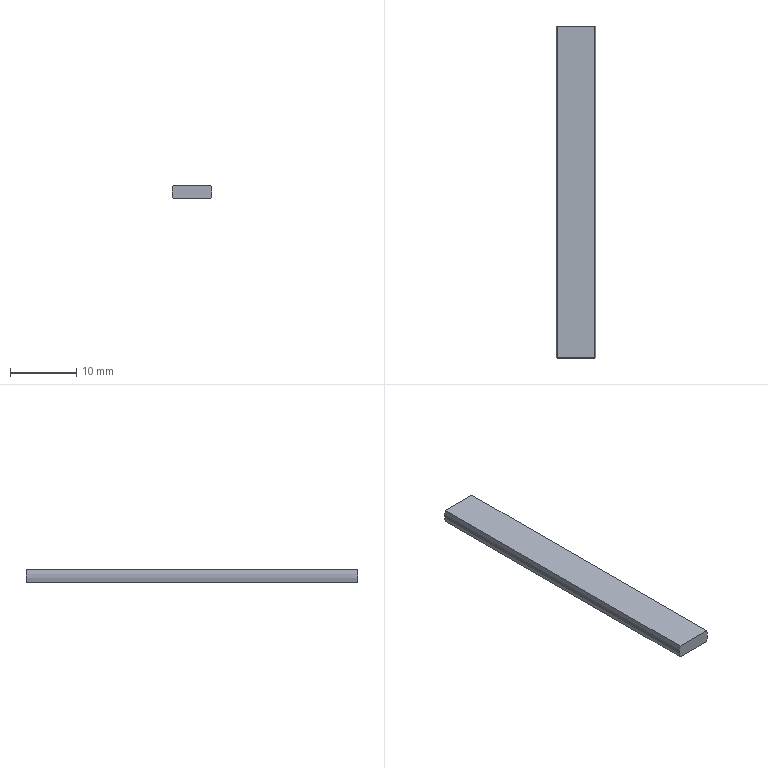Part | STEP file | Cooling fin - Tower - 1 cav | 1 solid | 6 faces | box 6 x 50 x 2 mm | volume 588.696 mm3 | plane 4 | cylinder 2 | commonest cylinder face diameters 6 x2
STEP:
#1=CARTESIAN_POINT('',(0.,0.,0.));
#2=DIRECTION('',(0.,0.,1.));
#3=DIRECTION('',(1.,0.,0.));
#4=AXIS2_PLACEMENT_3D('',#1,#2,#3);
#5=CARTESIAN_POINT('',(2.828,0.,-1.));
#6=VERTEX_POINT('',#5);
#7=CARTESIAN_POINT('',(2.828,50.,-1.));
#8=VERTEX_POINT('',#7);
#9=CARTESIAN_POINT('',(2.828,0.,-1.));
#10=DIRECTION('',(0.,1.,0.));
#11=VECTOR('',#10,1.);
#12=LINE('',#9,#11);
#13=CARTESIAN_POINT('',(-5.,50.,-1.));
#14=DIRECTION('',(0.,0.,1.));
#15=DIRECTION('',(1.,0.,0.));
#16=AXIS2_PLACEMENT_3D('',#13,#14,#15);
#17=PLANE('',#16);
#18=CARTESIAN_POINT('',(7.828,-50.));
#19=DIRECTION('',(0.,1.));
#20=VECTOR('',#19,1.);
#21=LINE('',#18,#20);
#22=(GEOMETRIC_REPRESENTATION_CONTEXT(2)PARAMETRIC_REPRESENTATION_CONTEXT()REPRESENTATION_CONTEXT('',''));
#23=DEFINITIONAL_REPRESENTATION('',(#21),#22);
#24=PCURVE('',#17,#23);
#25=CARTESIAN_POINT('',(0.,0.,0.));
#26=DIRECTION('',(0.,1.,0.));
#27=DIRECTION('',(0.,0.,1.));
#28=AXIS2_PLACEMENT_3D('',#25,#26,#27);
#29=CYLINDRICAL_SURFACE('',#28,3.);
#30=CARTESIAN_POINT('',(1.911,0.));
#31=DIRECTION('',(0.,1.));
#32=VECTOR('',#31,1.);
#33=LINE('',#30,#32);
#34=(GEOMETRIC_REPRESENTATION_CONTEXT(2)PARAMETRIC_REPRESENTATION_CONTEXT()REPRESENTATION_CONTEXT('',''));
#35=DEFINITIONAL_REPRESENTATION('',(#33),#34);
#36=PCURVE('',#29,#35);
#37=SURFACE_CURVE('',#12,(#24,#36),.PCURVE_S1.);
#38=EDGE_CURVE('',#6,#8,#37,.T.);
#39=ORIENTED_EDGE('',*,*,#38,.F.);
#40=CARTESIAN_POINT('',(-2.828,0.,-1.));
#41=VERTEX_POINT('',#40);
#42=CARTESIAN_POINT('',(-5.,0.,-1.));
#43=DIRECTION('',(-1.,0.,0.));
#44=VECTOR('',#43,1.);
#45=LINE('',#42,#44);
#46=CARTESIAN_POINT('',(0.,-50.));
#47=DIRECTION('',(-1.,0.));
#48=VECTOR('',#47,1.);
#49=LINE('',#46,#48);
#50=(GEOMETRIC_REPRESENTATION_CONTEXT(2)PARAMETRIC_REPRESENTATION_CONTEXT()REPRESENTATION_CONTEXT('',''));
#51=DEFINITIONAL_REPRESENTATION('',(#49),#50);
#52=PCURVE('',#17,#51);
#53=CARTESIAN_POINT('',(0.,0.,0.));
#54=DIRECTION('',(0.,-1.,0.));
#55=DIRECTION('',(0.,0.,-1.));
#56=AXIS2_PLACEMENT_3D('',#53,#54,#55);
#57=PLANE('',#56);
#58=CARTESIAN_POINT('',(1.,-5.));
#59=DIRECTION('',(0.,-1.));
#60=VECTOR('',#59,1.);
#61=LINE('',#58,#60);
#62=(GEOMETRIC_REPRESENTATION_CONTEXT(2)PARAMETRIC_REPRESENTATION_CONTEXT()REPRESENTATION_CONTEXT('',''));
#63=DEFINITIONAL_REPRESENTATION('',(#61),#62);
#64=PCURVE('',#57,#63);
#65=SURFACE_CURVE('',#45,(#52,#64),.PCURVE_S1.);
#66=EDGE_CURVE('',#6,#41,#65,.T.);
#67=ORIENTED_EDGE('',*,*,#66,.T.);
#68=CARTESIAN_POINT('',(-2.828,50.,-1.));
#69=VERTEX_POINT('',#68);
#70=CARTESIAN_POINT('',(-2.828,0.,-1.));
#71=DIRECTION('',(0.,-1.,0.));
#72=VECTOR('',#71,1.);
#73=LINE('',#70,#72);
#74=CARTESIAN_POINT('',(2.172,-50.));
#75=DIRECTION('',(0.,-1.));
#76=VECTOR('',#75,1.);
#77=LINE('',#74,#76);
#78=(GEOMETRIC_REPRESENTATION_CONTEXT(2)PARAMETRIC_REPRESENTATION_CONTEXT()REPRESENTATION_CONTEXT('',''));
#79=DEFINITIONAL_REPRESENTATION('',(#77),#78);
#80=PCURVE('',#17,#79);
#81=CARTESIAN_POINT('',(0.,0.,0.));
#82=DIRECTION('',(0.,1.,0.));
#83=DIRECTION('',(0.,0.,1.));
#84=AXIS2_PLACEMENT_3D('',#81,#82,#83);
#85=CYLINDRICAL_SURFACE('',#84,3.);
#86=CARTESIAN_POINT('',(4.373,0.));
#87=DIRECTION('',(0.,-1.));
#88=VECTOR('',#87,1.);
#89=LINE('',#86,#88);
#90=(GEOMETRIC_REPRESENTATION_CONTEXT(2)PARAMETRIC_REPRESENTATION_CONTEXT()REPRESENTATION_CONTEXT('',''));
#91=DEFINITIONAL_REPRESENTATION('',(#89),#90);
#92=PCURVE('',#85,#91);
#93=SURFACE_CURVE('',#73,(#80,#92),.PCURVE_S1.);
#94=EDGE_CURVE('',#69,#41,#93,.T.);
#95=ORIENTED_EDGE('',*,*,#94,.F.);
#96=CARTESIAN_POINT('',(-5.,50.,-1.));
#97=DIRECTION('',(-1.,0.,0.));
#98=VECTOR('',#97,1.);
#99=LINE('',#96,#98);
#100=CARTESIAN_POINT('',(0.,0.));
#101=DIRECTION('',(-1.,0.));
#102=VECTOR('',#101,1.);
#103=LINE('',#100,#102);
#104=(GEOMETRIC_REPRESENTATION_CONTEXT(2)PARAMETRIC_REPRESENTATION_CONTEXT()REPRESENTATION_CONTEXT('',''));
#105=DEFINITIONAL_REPRESENTATION('',(#103),#104);
#106=PCURVE('',#17,#105);
#107=CARTESIAN_POINT('',(0.,50.,0.));
#108=DIRECTION('',(0.,-1.,0.));
#109=DIRECTION('',(0.,0.,-1.));
#110=AXIS2_PLACEMENT_3D('',#107,#108,#109);
#111=PLANE('',#110);
#112=CARTESIAN_POINT('',(1.,-5.));
#113=DIRECTION('',(0.,-1.));
#114=VECTOR('',#113,1.);
#115=LINE('',#112,#114);
#116=(GEOMETRIC_REPRESENTATION_CONTEXT(2)PARAMETRIC_REPRESENTATION_CONTEXT()REPRESENTATION_CONTEXT('',''));
#117=DEFINITIONAL_REPRESENTATION('',(#115),#116);
#118=PCURVE('',#111,#117);
#119=SURFACE_CURVE('',#99,(#106,#118),.PCURVE_S1.);
#120=EDGE_CURVE('',#8,#69,#119,.T.);
#121=ORIENTED_EDGE('',*,*,#120,.F.);
#122=EDGE_LOOP('',(#39,#67,#95,#121));
#123=FACE_BOUND('',#122,.T.);
#124=ADVANCED_FACE('',(#123),#17,.F.);
#125=CARTESIAN_POINT('',(-2.828,0.,1.));
#126=VERTEX_POINT('',#125);
#127=CARTESIAN_POINT('',(-2.828,50.,1.));
#128=VERTEX_POINT('',#127);
#129=CARTESIAN_POINT('',(-2.828,0.,1.));
#130=DIRECTION('',(0.,1.,0.));
#131=VECTOR('',#130,1.);
#132=LINE('',#129,#131);
#133=CARTESIAN_POINT('',(-5.,50.,1.));
#134=DIRECTION('',(0.,0.,-1.));
#135=DIRECTION('',(-1.,0.,0.));
#136=AXIS2_PLACEMENT_3D('',#133,#134,#135);
#137=PLANE('',#136);
#138=CARTESIAN_POINT('',(-2.172,-50.));
#139=DIRECTION('',(0.,1.));
#140=VECTOR('',#139,1.);
#141=LINE('',#138,#140);
#142=(GEOMETRIC_REPRESENTATION_CONTEXT(2)PARAMETRIC_REPRESENTATION_CONTEXT()REPRESENTATION_CONTEXT('',''));
#143=DEFINITIONAL_REPRESENTATION('',(#141),#142);
#144=PCURVE('',#137,#143);
#145=CARTESIAN_POINT('',(5.052,0.));
#146=DIRECTION('',(0.,1.));
#147=VECTOR('',#146,1.);
#148=LINE('',#145,#147);
#149=(GEOMETRIC_REPRESENTATION_CONTEXT(2)PARAMETRIC_REPRESENTATION_CONTEXT()REPRESENTATION_CONTEXT('',''));
#150=DEFINITIONAL_REPRESENTATION('',(#148),#149);
#151=PCURVE('',#85,#150);
#152=SURFACE_CURVE('',#132,(#144,#151),.PCURVE_S1.);
#153=EDGE_CURVE('',#126,#128,#152,.T.);
#154=ORIENTED_EDGE('',*,*,#153,.F.);
#155=CARTESIAN_POINT('',(2.828,0.,1.));
#156=VERTEX_POINT('',#155);
#157=CARTESIAN_POINT('',(-5.,0.,1.));
#158=DIRECTION('',(1.,0.,0.));
#159=VECTOR('',#158,1.);
#160=LINE('',#157,#159);
#161=CARTESIAN_POINT('',(0.,-50.));
#162=DIRECTION('',(-1.,0.));
#163=VECTOR('',#162,1.);
#164=LINE('',#161,#163);
#165=(GEOMETRIC_REPRESENTATION_CONTEXT(2)PARAMETRIC_REPRESENTATION_CONTEXT()REPRESENTATION_CONTEXT('',''));
#166=DEFINITIONAL_REPRESENTATION('',(#164),#165);
#167=PCURVE('',#137,#166);
#168=CARTESIAN_POINT('',(-1.,-5.));
#169=DIRECTION('',(0.,1.));
#170=VECTOR('',#169,1.);
#171=LINE('',#168,#170);
#172=(GEOMETRIC_REPRESENTATION_CONTEXT(2)PARAMETRIC_REPRESENTATION_CONTEXT()REPRESENTATION_CONTEXT('',''));
#173=DEFINITIONAL_REPRESENTATION('',(#171),#172);
#174=PCURVE('',#57,#173);
#175=SURFACE_CURVE('',#160,(#167,#174),.PCURVE_S1.);
#176=EDGE_CURVE('',#126,#156,#175,.T.);
#177=ORIENTED_EDGE('',*,*,#176,.T.);
#178=CARTESIAN_POINT('',(2.828,50.,1.));
#179=VERTEX_POINT('',#178);
#180=CARTESIAN_POINT('',(2.828,0.,1.));
#181=DIRECTION('',(0.,-1.,0.));
#182=VECTOR('',#181,1.);
#183=LINE('',#180,#182);
#184=CARTESIAN_POINT('',(-7.828,-50.));
#185=DIRECTION('',(0.,-1.));
#186=VECTOR('',#185,1.);
#187=LINE('',#184,#186);
#188=(GEOMETRIC_REPRESENTATION_CONTEXT(2)PARAMETRIC_REPRESENTATION_CONTEXT()REPRESENTATION_CONTEXT('',''));
#189=DEFINITIONAL_REPRESENTATION('',(#187),#188);
#190=PCURVE('',#137,#189);
#191=CARTESIAN_POINT('',(1.231,0.));
#192=DIRECTION('',(0.,-1.));
#193=VECTOR('',#192,1.);
#194=LINE('',#191,#193);
#195=(GEOMETRIC_REPRESENTATION_CONTEXT(2)PARAMETRIC_REPRESENTATION_CONTEXT()REPRESENTATION_CONTEXT('',''));
#196=DEFINITIONAL_REPRESENTATION('',(#194),#195);
#197=PCURVE('',#29,#196);
#198=SURFACE_CURVE('',#183,(#190,#197),.PCURVE_S1.);
#199=EDGE_CURVE('',#179,#156,#198,.T.);
#200=ORIENTED_EDGE('',*,*,#199,.F.);
#201=CARTESIAN_POINT('',(-5.,50.,1.));
#202=DIRECTION('',(1.,0.,0.));
#203=VECTOR('',#202,1.);
#204=LINE('',#201,#203);
#205=CARTESIAN_POINT('',(0.,0.));
#206=DIRECTION('',(-1.,0.));
#207=VECTOR('',#206,1.);
#208=LINE('',#205,#207);
#209=(GEOMETRIC_REPRESENTATION_CONTEXT(2)PARAMETRIC_REPRESENTATION_CONTEXT()REPRESENTATION_CONTEXT('',''));
#210=DEFINITIONAL_REPRESENTATION('',(#208),#209);
#211=PCURVE('',#137,#210);
#212=CARTESIAN_POINT('',(-1.,-5.));
#213=DIRECTION('',(0.,1.));
#214=VECTOR('',#213,1.);
#215=LINE('',#212,#214);
#216=(GEOMETRIC_REPRESENTATION_CONTEXT(2)PARAMETRIC_REPRESENTATION_CONTEXT()REPRESENTATION_CONTEXT('',''));
#217=DEFINITIONAL_REPRESENTATION('',(#215),#216);
#218=PCURVE('',#111,#217);
#219=SURFACE_CURVE('',#204,(#211,#218),.PCURVE_S1.);
#220=EDGE_CURVE('',#128,#179,#219,.T.);
#221=ORIENTED_EDGE('',*,*,#220,.F.);
#222=EDGE_LOOP('',(#154,#177,#200,#221));
#223=FACE_BOUND('',#222,.T.);
#224=ADVANCED_FACE('',(#223),#137,.F.);
#225=CARTESIAN_POINT('',(0.,50.,0.));
#226=DIRECTION('',(0.,1.,0.));
#227=DIRECTION('',(0.,0.,1.));
#228=AXIS2_PLACEMENT_3D('',#225,#226,#227);
#229=CIRCLE('',#228,3.);
#230=CARTESIAN_POINT('',(-3.,0.));
#231=CARTESIAN_POINT('',(-3.,5.196));
#232=CARTESIAN_POINT('',(1.5,2.598));
#233=CARTESIAN_POINT('',(6.,0.));
#234=CARTESIAN_POINT('',(1.5,-2.598));
#235=CARTESIAN_POINT('',(-3.,-5.196));
#236=CARTESIAN_POINT('',(-3.,0.));
#237=(BOUNDED_CURVE()B_SPLINE_CURVE(2,(#230,#231,#232,#233,#234,#235,#236),.UNSPECIFIED.,.T.,.F.)B_SPLINE_CURVE_WITH_KNOTS((1,2,2,2,2,1),(-2.094,0.,2.094,4.189,6.283,8.378),.UNSPECIFIED.)CURVE()GEOMETRIC_REPRESENTATION_ITEM()RATIONAL_B_SPLINE_CURVE((1.,0.5,1.,0.5,1.,0.5,1.))REPRESENTATION_ITEM(''));
#238=(GEOMETRIC_REPRESENTATION_CONTEXT(2)PARAMETRIC_REPRESENTATION_CONTEXT()REPRESENTATION_CONTEXT('',''));
#239=DEFINITIONAL_REPRESENTATION('',(#237),#238);
#240=PCURVE('',#111,#239);
#241=CARTESIAN_POINT('',(0.,50.));
#242=DIRECTION('',(1.,0.));
#243=VECTOR('',#242,1.);
#244=LINE('',#241,#243);
#245=(GEOMETRIC_REPRESENTATION_CONTEXT(2)PARAMETRIC_REPRESENTATION_CONTEXT()REPRESENTATION_CONTEXT('',''));
#246=DEFINITIONAL_REPRESENTATION('',(#244),#245);
#247=PCURVE('',#29,#246);
#248=SURFACE_CURVE('',#229,(#240,#247),.PCURVE_S1.);
#249=EDGE_CURVE('',#179,#8,#248,.T.);
#250=ORIENTED_EDGE('',*,*,#249,.T.);
#251=ORIENTED_EDGE('',*,*,#120,.T.);
#252=CARTESIAN_POINT('',(0.,50.,0.));
#253=DIRECTION('',(0.,1.,0.));
#254=DIRECTION('',(0.,0.,1.));
#255=AXIS2_PLACEMENT_3D('',#252,#253,#254);
#256=CIRCLE('',#255,3.);
#257=CARTESIAN_POINT('',(-3.,0.));
#258=CARTESIAN_POINT('',(-3.,5.196));
#259=CARTESIAN_POINT('',(1.5,2.598));
#260=CARTESIAN_POINT('',(6.,0.));
#261=CARTESIAN_POINT('',(1.5,-2.598));
#262=CARTESIAN_POINT('',(-3.,-5.196));
#263=CARTESIAN_POINT('',(-3.,0.));
#264=(BOUNDED_CURVE()B_SPLINE_CURVE(2,(#257,#258,#259,#260,#261,#262,#263),.UNSPECIFIED.,.T.,.F.)B_SPLINE_CURVE_WITH_KNOTS((1,2,2,2,2,1),(-2.094,0.,2.094,4.189,6.283,8.378),.UNSPECIFIED.)CURVE()GEOMETRIC_REPRESENTATION_ITEM()RATIONAL_B_SPLINE_CURVE((1.,0.5,1.,0.5,1.,0.5,1.))REPRESENTATION_ITEM(''));
#265=(GEOMETRIC_REPRESENTATION_CONTEXT(2)PARAMETRIC_REPRESENTATION_CONTEXT()REPRESENTATION_CONTEXT('',''));
#266=DEFINITIONAL_REPRESENTATION('',(#264),#265);
#267=PCURVE('',#111,#266);
#268=CARTESIAN_POINT('',(0.,50.));
#269=DIRECTION('',(1.,0.));
#270=VECTOR('',#269,1.);
#271=LINE('',#268,#270);
#272=(GEOMETRIC_REPRESENTATION_CONTEXT(2)PARAMETRIC_REPRESENTATION_CONTEXT()REPRESENTATION_CONTEXT('',''));
#273=DEFINITIONAL_REPRESENTATION('',(#271),#272);
#274=PCURVE('',#85,#273);
#275=SURFACE_CURVE('',#256,(#267,#274),.PCURVE_S1.);
#276=EDGE_CURVE('',#69,#128,#275,.T.);
#277=ORIENTED_EDGE('',*,*,#276,.T.);
#278=ORIENTED_EDGE('',*,*,#220,.T.);
#279=EDGE_LOOP('',(#250,#251,#277,#278));
#280=FACE_BOUND('',#279,.T.);
#281=ADVANCED_FACE('',(#280),#111,.F.);
#282=ORIENTED_EDGE('',*,*,#66,.F.);
#283=CARTESIAN_POINT('',(0.,0.,0.));
#284=DIRECTION('',(0.,1.,0.));
#285=DIRECTION('',(0.,0.,1.));
#286=AXIS2_PLACEMENT_3D('',#283,#284,#285);
#287=CIRCLE('',#286,3.);
#288=CARTESIAN_POINT('',(-3.,0.));
#289=CARTESIAN_POINT('',(-3.,5.196));
#290=CARTESIAN_POINT('',(1.5,2.598));
#291=CARTESIAN_POINT('',(6.,0.));
#292=CARTESIAN_POINT('',(1.5,-2.598));
#293=CARTESIAN_POINT('',(-3.,-5.196));
#294=CARTESIAN_POINT('',(-3.,0.));
#295=(BOUNDED_CURVE()B_SPLINE_CURVE(2,(#288,#289,#290,#291,#292,#293,#294),.UNSPECIFIED.,.T.,.F.)B_SPLINE_CURVE_WITH_KNOTS((1,2,2,2,2,1),(-2.094,0.,2.094,4.189,6.283,8.378),.UNSPECIFIED.)CURVE()GEOMETRIC_REPRESENTATION_ITEM()RATIONAL_B_SPLINE_CURVE((1.,0.5,1.,0.5,1.,0.5,1.))REPRESENTATION_ITEM(''));
#296=(GEOMETRIC_REPRESENTATION_CONTEXT(2)PARAMETRIC_REPRESENTATION_CONTEXT()REPRESENTATION_CONTEXT('',''));
#297=DEFINITIONAL_REPRESENTATION('',(#295),#296);
#298=PCURVE('',#57,#297);
#299=CARTESIAN_POINT('',(0.,0.));
#300=DIRECTION('',(1.,0.));
#301=VECTOR('',#300,1.);
#302=LINE('',#299,#301);
#303=(GEOMETRIC_REPRESENTATION_CONTEXT(2)PARAMETRIC_REPRESENTATION_CONTEXT()REPRESENTATION_CONTEXT('',''));
#304=DEFINITIONAL_REPRESENTATION('',(#302),#303);
#305=PCURVE('',#29,#304);
#306=SURFACE_CURVE('',#287,(#298,#305),.PCURVE_S1.);
#307=EDGE_CURVE('',#156,#6,#306,.T.);
#308=ORIENTED_EDGE('',*,*,#307,.F.);
#309=ORIENTED_EDGE('',*,*,#176,.F.);
#310=CARTESIAN_POINT('',(0.,0.,0.));
#311=DIRECTION('',(0.,-1.,0.));
#312=DIRECTION('',(0.,0.,-1.));
#313=AXIS2_PLACEMENT_3D('',#310,#311,#312);
#314=CIRCLE('',#313,3.);
#315=CARTESIAN_POINT('',(0.,0.));
#316=DIRECTION('',(1.,0.));
#317=AXIS2_PLACEMENT_2D('',#315,#316);
#318=CIRCLE('',#317,3.);
#319=(GEOMETRIC_REPRESENTATION_CONTEXT(2)PARAMETRIC_REPRESENTATION_CONTEXT()REPRESENTATION_CONTEXT('',''));
#320=DEFINITIONAL_REPRESENTATION('',(#318),#319);
#321=PCURVE('',#57,#320);
#322=CARTESIAN_POINT('',(9.425,0.));
#323=DIRECTION('',(-1.,0.));
#324=VECTOR('',#323,1.);
#325=LINE('',#322,#324);
#326=(GEOMETRIC_REPRESENTATION_CONTEXT(2)PARAMETRIC_REPRESENTATION_CONTEXT()REPRESENTATION_CONTEXT('',''));
#327=DEFINITIONAL_REPRESENTATION('',(#325),#326);
#328=PCURVE('',#85,#327);
#329=SURFACE_CURVE('',#314,(#321,#328),.PCURVE_S1.);
#330=EDGE_CURVE('',#126,#41,#329,.T.);
#331=ORIENTED_EDGE('',*,*,#330,.T.);
#332=EDGE_LOOP('',(#282,#308,#309,#331));
#333=FACE_BOUND('',#332,.T.);
#334=ADVANCED_FACE('',(#333),#57,.T.);
#335=ORIENTED_EDGE('',*,*,#94,.T.);
#336=ORIENTED_EDGE('',*,*,#330,.F.);
#337=ORIENTED_EDGE('',*,*,#153,.T.);
#338=ORIENTED_EDGE('',*,*,#276,.F.);
#339=EDGE_LOOP('',(#335,#336,#337,#338));
#340=FACE_BOUND('',#339,.T.);
#341=ADVANCED_FACE('',(#340),#85,.T.);
#342=ORIENTED_EDGE('',*,*,#38,.T.);
#343=ORIENTED_EDGE('',*,*,#249,.F.);
#344=ORIENTED_EDGE('',*,*,#199,.T.);
#345=ORIENTED_EDGE('',*,*,#307,.T.);
#346=EDGE_LOOP('',(#342,#343,#344,#345));
#347=FACE_BOUND('',#346,.T.);
#348=ADVANCED_FACE('',(#347),#29,.T.);
#349=CLOSED_SHELL('',(#124,#224,#281,#334,#341,#348));
#350=MANIFOLD_SOLID_BREP('',#349);
#351=(LENGTH_UNIT()NAMED_UNIT(*)SI_UNIT(.MILLI.,.METRE.));
#352=UNCERTAINTY_MEASURE_WITH_UNIT(LENGTH_MEASURE(0.0000001),#351,'','');
#353=(NAMED_UNIT(*)PLANE_ANGLE_UNIT()SI_UNIT($,.RADIAN.));
#354=(NAMED_UNIT(*)SI_UNIT($,.STERADIAN.)SOLID_ANGLE_UNIT());
#355=(GEOMETRIC_REPRESENTATION_CONTEXT(3)GLOBAL_UNCERTAINTY_ASSIGNED_CONTEXT((#352))GLOBAL_UNIT_ASSIGNED_CONTEXT((#351,#353,#354))REPRESENTATION_CONTEXT('',''));
#356=ADVANCED_BREP_SHAPE_REPRESENTATION('',(#4,#350),#355);